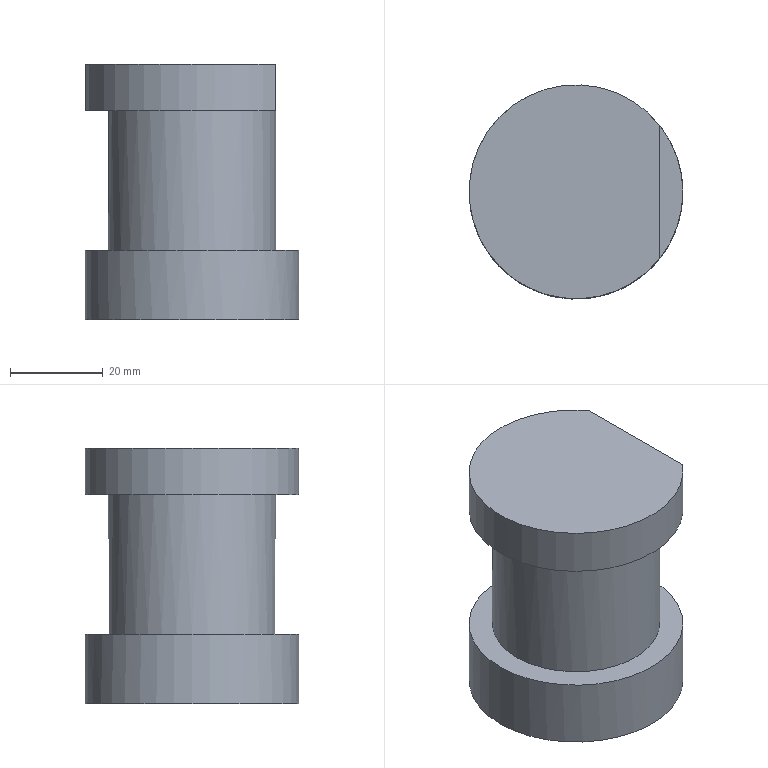Part | NX | features solid 2 | 1 solid | 11 faces | box 46 x 46 x 55 mm | volume 61296 mm3 | plane 5 | cylinder 4 | cone 2 | commonest cylinder face diameters 46 x2 16 x1 36 x1
STEP:
#1=CARTESIAN_POINT('',(253.,264.318,95.));
#2=VERTEX_POINT('',#1);
#3=CARTESIAN_POINT('',(253.,235.682,95.));
#4=VERTEX_POINT('',#3);
#5=CARTESIAN_POINT('',(235.,250.,95.));
#6=DIRECTION('',(0.,0.,1.));
#7=DIRECTION('',(1.,0.,0.));
#8=AXIS2_PLACEMENT_3D('',#5,#6,#7);
#9=CIRCLE('',#8,23.);
#10=EDGE_CURVE('',#2,#4,#9,.T.);
#11=ORIENTED_EDGE('',*,*,#10,.T.);
#12=CARTESIAN_POINT('',(253.,235.682,105.));
#13=VERTEX_POINT('',#12);
#14=CARTESIAN_POINT('',(253.,235.682,110.));
#15=DIRECTION('',(0.,0.,-1.));
#16=VECTOR('',#15,1000.);
#17=LINE('',#14,#16);
#18=EDGE_CURVE('',#13,#4,#17,.T.);
#19=ORIENTED_EDGE('',*,*,#18,.F.);
#20=CARTESIAN_POINT('',(253.,264.318,105.));
#21=VERTEX_POINT('',#20);
#22=CARTESIAN_POINT('',(235.,250.,105.));
#23=DIRECTION('',(0.,0.,-1.));
#24=DIRECTION('',(-1.,0.,0.));
#25=AXIS2_PLACEMENT_3D('',#22,#23,#24);
#26=CIRCLE('',#25,23.);
#27=EDGE_CURVE('',#13,#21,#26,.T.);
#28=ORIENTED_EDGE('',*,*,#27,.T.);
#29=CARTESIAN_POINT('',(253.,264.318,110.));
#30=DIRECTION('',(0.,0.,-1.));
#31=VECTOR('',#30,1000.);
#32=LINE('',#29,#31);
#33=EDGE_CURVE('',#2,#21,#32,.F.);
#34=ORIENTED_EDGE('',*,*,#33,.F.);
#35=EDGE_LOOP('',(#11,#19,#28,#34));
#36=FACE_BOUND('',#35,.T.);
#37=CARTESIAN_POINT('',(235.,250.,105.));
#38=DIRECTION('',(0.,0.,-1.));
#39=DIRECTION('',(-1.,0.,0.));
#40=AXIS2_PLACEMENT_3D('',#37,#38,#39);
#41=CYLINDRICAL_SURFACE('',#40,23.);
#42=ADVANCED_FACE('',(#36),#41,.T.);
#43=CARTESIAN_POINT('',(253.,250.,105.));
#44=DIRECTION('',(0.,-1.,0.));
#45=VECTOR('',#44,1000.);
#46=LINE('',#43,#45);
#47=EDGE_CURVE('',#21,#13,#46,.T.);
#48=ORIENTED_EDGE('',*,*,#47,.F.);
#49=ORIENTED_EDGE('',*,*,#27,.F.);
#50=EDGE_LOOP('',(#48,#49));
#51=FACE_BOUND('',#50,.T.);
#52=CARTESIAN_POINT('',(235.,250.,105.));
#53=DIRECTION('',(0.,0.,-1.));
#54=DIRECTION('',(-1.,0.,0.));
#55=AXIS2_PLACEMENT_3D('',#52,#53,#54);
#56=PLANE('',#55);
#57=ADVANCED_FACE('',(#51),#56,.F.);
#58=ORIENTED_EDGE('',*,*,#10,.F.);
#59=CARTESIAN_POINT('',(253.,250.,95.));
#60=VERTEX_POINT('',#59);
#61=CARTESIAN_POINT('',(253.,264.318,95.));
#62=DIRECTION('',(0.,-1.,0.));
#63=VECTOR('',#62,1000.);
#64=LINE('',#61,#63);
#65=EDGE_CURVE('',#2,#60,#64,.T.);
#66=ORIENTED_EDGE('',*,*,#65,.T.);
#67=CARTESIAN_POINT('',(235.,250.,95.));
#68=DIRECTION('',(0.,0.,-1.));
#69=DIRECTION('',(-1.,0.,0.));
#70=AXIS2_PLACEMENT_3D('',#67,#68,#69);
#71=CIRCLE('',#70,18.);
#72=EDGE_CURVE('',#60,#60,#71,.T.);
#73=ORIENTED_EDGE('',*,*,#72,.F.);
#74=CARTESIAN_POINT('',(253.,264.318,95.));
#75=DIRECTION('',(0.,-1.,0.));
#76=VECTOR('',#75,1000.);
#77=LINE('',#74,#76);
#78=EDGE_CURVE('',#60,#4,#77,.T.);
#79=ORIENTED_EDGE('',*,*,#78,.T.);
#80=EDGE_LOOP('',(#58,#66,#73,#79));
#81=FACE_BOUND('',#80,.T.);
#82=CARTESIAN_POINT('',(235.,250.,95.));
#83=DIRECTION('',(0.,0.,1.));
#84=DIRECTION('',(1.,0.,0.));
#85=AXIS2_PLACEMENT_3D('',#82,#83,#84);
#86=PLANE('',#85);
#87=ADVANCED_FACE('',(#81),#86,.F.);
#88=CARTESIAN_POINT('',(258.,250.,65.));
#89=VERTEX_POINT('',#88);
#90=CARTESIAN_POINT('',(235.,250.,65.));
#91=DIRECTION('',(0.,0.,1.));
#92=DIRECTION('',(1.,0.,0.));
#93=AXIS2_PLACEMENT_3D('',#90,#91,#92);
#94=CIRCLE('',#93,23.);
#95=EDGE_CURVE('',#89,#89,#94,.F.);
#96=ORIENTED_EDGE('',*,*,#95,.F.);
#97=EDGE_LOOP('',(#96));
#98=FACE_BOUND('',#97,.T.);
#99=CARTESIAN_POINT('',(217.,250.,65.));
#100=VERTEX_POINT('',#99);
#101=CARTESIAN_POINT('',(235.,250.,65.));
#102=DIRECTION('',(0.,0.,-1.));
#103=DIRECTION('',(-1.,0.,0.));
#104=AXIS2_PLACEMENT_3D('',#101,#102,#103);
#105=CIRCLE('',#104,18.);
#106=EDGE_CURVE('',#100,#100,#105,.T.);
#107=ORIENTED_EDGE('',*,*,#106,.T.);
#108=EDGE_LOOP('',(#107));
#109=FACE_BOUND('',#108,.T.);
#110=CARTESIAN_POINT('',(235.,250.,65.));
#111=DIRECTION('',(0.,0.,1.));
#112=DIRECTION('',(1.,0.,0.));
#113=AXIS2_PLACEMENT_3D('',#110,#111,#112);
#114=PLANE('',#113);
#115=ADVANCED_FACE('',(#98,#109),#114,.T.);
#116=ORIENTED_EDGE('',*,*,#72,.T.);
#117=EDGE_LOOP('',(#116));
#118=FACE_BOUND('',#117,.T.);
#119=ORIENTED_EDGE('',*,*,#106,.F.);
#120=EDGE_LOOP('',(#119));
#121=FACE_BOUND('',#120,.T.);
#122=CARTESIAN_POINT('',(235.,250.,65.));
#123=DIRECTION('',(0.,0.,1.));
#124=DIRECTION('',(1.,0.,0.));
#125=AXIS2_PLACEMENT_3D('',#122,#123,#124);
#126=CYLINDRICAL_SURFACE('',#125,18.);
#127=ADVANCED_FACE('',(#118,#121),#126,.T.);
#128=CARTESIAN_POINT('',(224.,250.,50.));
#129=VERTEX_POINT('',#128);
#130=CARTESIAN_POINT('',(235.,250.,50.));
#131=DIRECTION('',(0.,0.,-1.));
#132=DIRECTION('',(-1.,0.,0.));
#133=AXIS2_PLACEMENT_3D('',#130,#131,#132);
#134=CIRCLE('',#133,11.);
#135=EDGE_CURVE('',#129,#129,#134,.T.);
#136=ORIENTED_EDGE('',*,*,#135,.F.);
#137=EDGE_LOOP('',(#136));
#138=FACE_BOUND('',#137,.T.);
#139=CARTESIAN_POINT('',(212.,250.,50.));
#140=VERTEX_POINT('',#139);
#141=CARTESIAN_POINT('',(235.,250.,50.));
#142=DIRECTION('',(0.,0.,-1.));
#143=DIRECTION('',(-1.,0.,0.));
#144=AXIS2_PLACEMENT_3D('',#141,#142,#143);
#145=CIRCLE('',#144,23.);
#146=EDGE_CURVE('',#140,#140,#145,.T.);
#147=ORIENTED_EDGE('',*,*,#146,.T.);
#148=EDGE_LOOP('',(#147));
#149=FACE_BOUND('',#148,.T.);
#150=CARTESIAN_POINT('',(235.,250.,50.));
#151=DIRECTION('',(0.,0.,-1.));
#152=DIRECTION('',(-1.,0.,0.));
#153=AXIS2_PLACEMENT_3D('',#150,#151,#152);
#154=PLANE('',#153);
#155=ADVANCED_FACE('',(#138,#149),#154,.T.);
#156=ORIENTED_EDGE('',*,*,#146,.F.);
#157=EDGE_LOOP('',(#156));
#158=FACE_BOUND('',#157,.T.);
#159=ORIENTED_EDGE('',*,*,#95,.T.);
#160=EDGE_LOOP('',(#159));
#161=FACE_BOUND('',#160,.T.);
#162=CARTESIAN_POINT('',(235.,250.,105.));
#163=DIRECTION('',(0.,0.,-1.));
#164=DIRECTION('',(-1.,0.,0.));
#165=AXIS2_PLACEMENT_3D('',#162,#163,#164);
#166=CYLINDRICAL_SURFACE('',#165,23.);
#167=ADVANCED_FACE('',(#158,#161),#166,.T.);
#168=ORIENTED_EDGE('',*,*,#135,.T.);
#169=EDGE_LOOP('',(#168));
#170=FACE_BOUND('',#169,.T.);
#171=CARTESIAN_POINT('',(227.,250.,55.196));
#172=VERTEX_POINT('',#171);
#173=CARTESIAN_POINT('',(235.,250.,55.196));
#174=DIRECTION('',(0.,0.,-1.));
#175=DIRECTION('',(-1.,0.,0.));
#176=AXIS2_PLACEMENT_3D('',#173,#174,#175);
#177=CIRCLE('',#176,8.);
#178=EDGE_CURVE('',#172,#172,#177,.T.);
#179=ORIENTED_EDGE('',*,*,#178,.F.);
#180=EDGE_LOOP('',(#179));
#181=FACE_BOUND('',#180,.T.);
#182=CARTESIAN_POINT('',(235.,250.,50.));
#183=DIRECTION('',(0.,0.,-1.));
#184=DIRECTION('',(1.,0.,0.));
#185=AXIS2_PLACEMENT_3D('',#182,#183,#184);
#186=CONICAL_SURFACE('',#185,11.,0.5236);
#187=ADVANCED_FACE('',(#170,#181),#186,.F.);
#188=CARTESIAN_POINT('',(243.,250.,95.));
#189=VERTEX_POINT('',#188);
#190=CARTESIAN_POINT('',(235.,250.,95.));
#191=DIRECTION('',(0.,0.,1.));
#192=DIRECTION('',(1.,0.,0.));
#193=AXIS2_PLACEMENT_3D('',#190,#191,#192);
#194=CIRCLE('',#193,8.);
#195=EDGE_CURVE('',#189,#189,#194,.T.);
#196=ORIENTED_EDGE('',*,*,#195,.F.);
#197=EDGE_LOOP('',(#196));
#198=FACE_BOUND('',#197,.T.);
#199=CARTESIAN_POINT('',(235.,250.,99.807));
#200=VERTEX_POINT('',#199);
#201=VERTEX_LOOP('',#200);
#202=FACE_BOUND('',#201,.T.);
#203=CARTESIAN_POINT('',(235.,250.,95.));
#204=DIRECTION('',(0.,0.,-1.));
#205=DIRECTION('',(-1.,0.,0.));
#206=AXIS2_PLACEMENT_3D('',#203,#204,#205);
#207=CONICAL_SURFACE('',#206,8.,1.03);
#208=ADVANCED_FACE('',(#198,#202),#207,.F.);
#209=ORIENTED_EDGE('',*,*,#178,.T.);
#210=EDGE_LOOP('',(#209));
#211=FACE_BOUND('',#210,.T.);
#212=ORIENTED_EDGE('',*,*,#195,.T.);
#213=EDGE_LOOP('',(#212));
#214=FACE_BOUND('',#213,.T.);
#215=CARTESIAN_POINT('',(235.,250.,50.));
#216=DIRECTION('',(0.,0.,1.));
#217=DIRECTION('',(1.,0.,0.));
#218=AXIS2_PLACEMENT_3D('',#215,#216,#217);
#219=CYLINDRICAL_SURFACE('',#218,8.);
#220=ADVANCED_FACE('',(#211,#214),#219,.F.);
#221=ORIENTED_EDGE('',*,*,#47,.T.);
#222=ORIENTED_EDGE('',*,*,#18,.T.);
#223=ORIENTED_EDGE('',*,*,#78,.F.);
#224=ORIENTED_EDGE('',*,*,#65,.F.);
#225=ORIENTED_EDGE('',*,*,#33,.T.);
#226=EDGE_LOOP('',(#221,#222,#223,#224,#225));
#227=FACE_BOUND('',#226,.T.);
#228=CARTESIAN_POINT('',(253.,264.318,110.));
#229=DIRECTION('',(1.,0.,0.));
#230=DIRECTION('',(0.,0.,-1.));
#231=AXIS2_PLACEMENT_3D('',#228,#229,#230);
#232=PLANE('',#231);
#233=ADVANCED_FACE('',(#227),#232,.T.);
#234=CLOSED_SHELL('',(#42,#57,#87,#115,#127,#155,#167,#187,#208,#220,#233));
#235=MANIFOLD_SOLID_BREP('',#234);
#236=(LENGTH_UNIT()NAMED_UNIT(*)SI_UNIT(.MILLI.,.METRE.));
#237=UNCERTAINTY_MEASURE_WITH_UNIT(LENGTH_MEASURE(0.00001),#236,'','');
#238=(NAMED_UNIT(*)PLANE_ANGLE_UNIT()SI_UNIT($,.RADIAN.));
#239=(NAMED_UNIT(*)SI_UNIT($,.STERADIAN.)SOLID_ANGLE_UNIT());
#240=(GEOMETRIC_REPRESENTATION_CONTEXT(3)GLOBAL_UNCERTAINTY_ASSIGNED_CONTEXT((#237))GLOBAL_UNIT_ASSIGNED_CONTEXT((#236,#238,#239))REPRESENTATION_CONTEXT('',''));
#241=ADVANCED_BREP_SHAPE_REPRESENTATION('',(#235),#240);